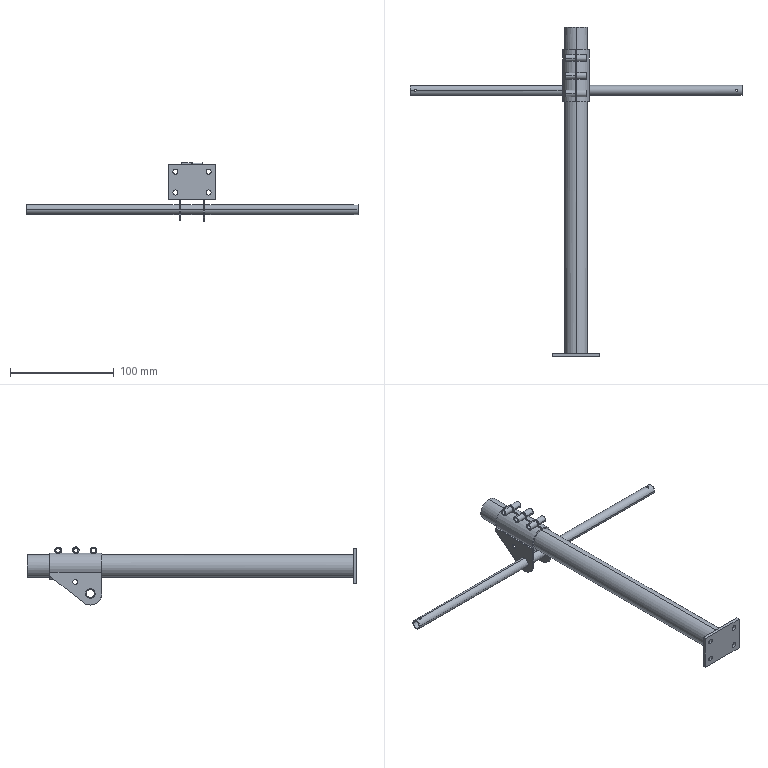Part | SolidWorks | features BaseBody 2 | 2 solids | 92 faces | box 320 x 318 x 55.956 mm | volume 42888 mm3 | cylinder 60 | plane 32 | commonest cylinder face diameters 4.2 x12 6.35 x12 2 x8 4.9 x8 9.5 x6 22 x5